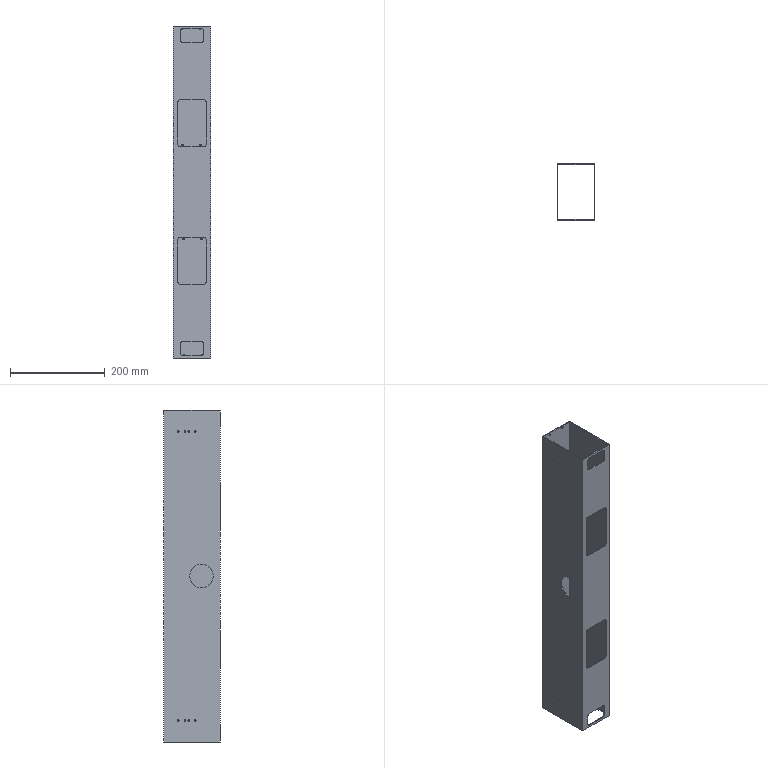Part | SolidWorks | features HoleWzd 4, ICE 2, Cut 1, ExtruThin 1, Fillet 1, MoveFace 1 | 1 solid | 76 faces | box 80 x 120 x 700 mm | volume 514821 mm3 | cylinder 50 | plane 26 | commonest cylinder face diameters 3.3 x16 3.6 x16 12 x16 50 x2